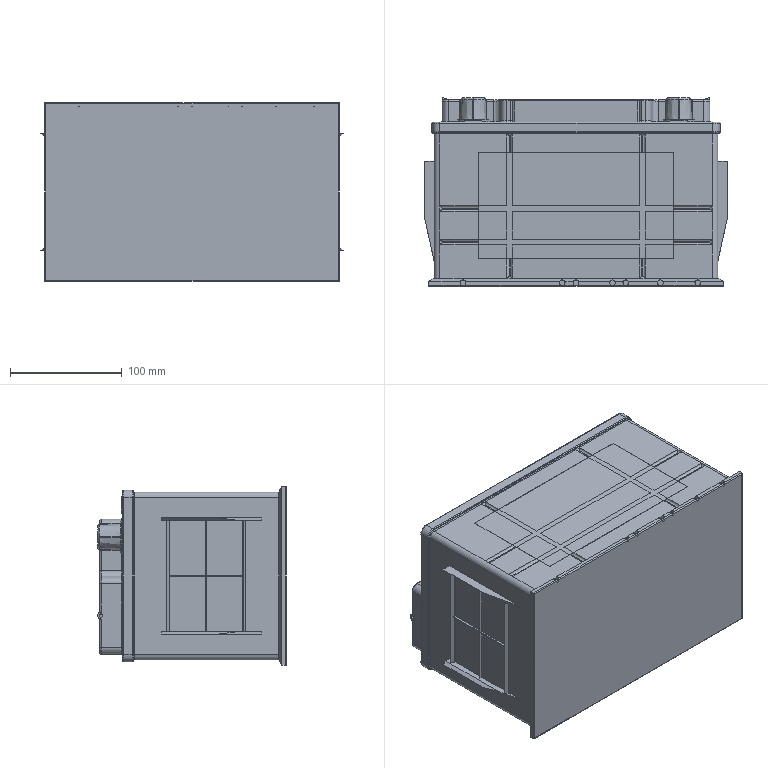Part | SolidWorks | features ICE 22, Fillet 10, Chamfer 4, Blend 3, MirrorPattern 3, CirPattern 2, Extrusion 1 | 1 solid | 526 faces | box 270.928 x 169.188 x 160 mm | volume 6109502 mm3 | plane 262 | cylinder 190 | torus 41 | cone 16 | sphere 11 | spline 6 | commonest cylinder face diameters 2 x80 4 x66 5 x14 12 x8 3.202 x4 10 x4